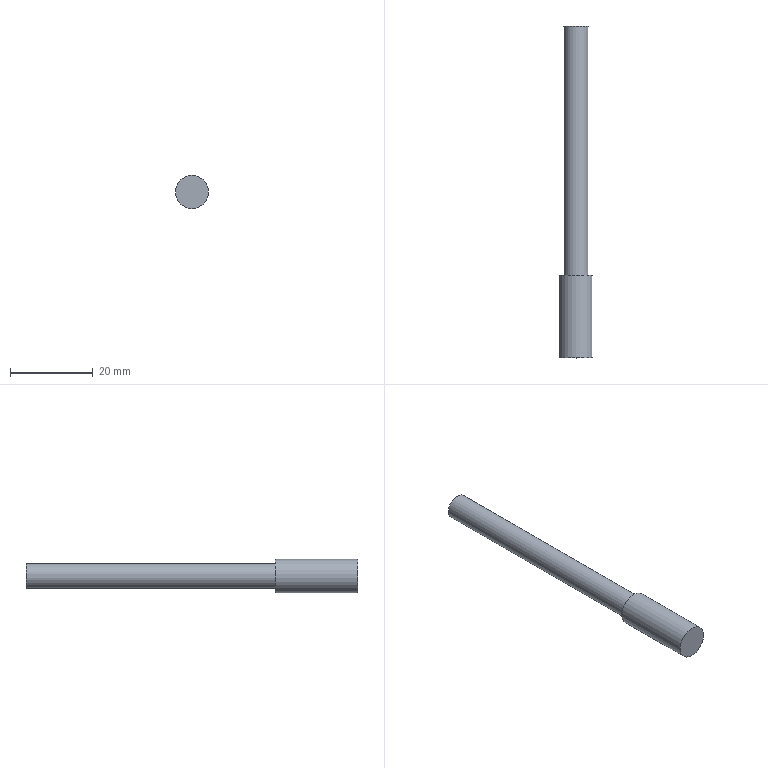Part | NX | features solid 2 | 1 solid | 5 faces | box 8 x 80 x 8 mm | volume 2700 mm3 | plane 3 | cylinder 2 | commonest cylinder face diameters 6 x1 8 x1
STEP:
#1=CARTESIAN_POINT('',(63.5,29.5,7.));
#2=VERTEX_POINT('',#1);
#3=CARTESIAN_POINT('',(63.5,29.5,4.));
#4=DIRECTION('',(0.,1.,0.));
#5=DIRECTION('',(0.,0.,1.));
#6=AXIS2_PLACEMENT_3D('',#3,#4,#5);
#7=CIRCLE('',#6,3.);
#8=EDGE_CURVE('',#2,#2,#7,.F.);
#9=ORIENTED_EDGE('',*,*,#8,.T.);
#10=EDGE_LOOP('',(#9));
#11=FACE_BOUND('',#10,.T.);
#12=CARTESIAN_POINT('',(63.5,-30.6,1.));
#13=VERTEX_POINT('',#12);
#14=CARTESIAN_POINT('',(63.5,-30.6,4.));
#15=DIRECTION('',(0.,-1.,0.));
#16=DIRECTION('',(0.,0.,-1.));
#17=AXIS2_PLACEMENT_3D('',#14,#15,#16);
#18=CIRCLE('',#17,3.);
#19=EDGE_CURVE('',#13,#13,#18,.F.);
#20=ORIENTED_EDGE('',*,*,#19,.T.);
#21=EDGE_LOOP('',(#20));
#22=FACE_BOUND('',#21,.T.);
#23=CARTESIAN_POINT('',(63.5,-69.,4.));
#24=DIRECTION('',(0.,1.,0.));
#25=DIRECTION('',(1.,0.,0.));
#26=AXIS2_PLACEMENT_3D('',#23,#24,#25);
#27=CYLINDRICAL_SURFACE('',#26,3.);
#28=ADVANCED_FACE('',(#11,#22),#27,.T.);
#29=ORIENTED_EDGE('',*,*,#8,.F.);
#30=EDGE_LOOP('',(#29));
#31=FACE_BOUND('',#30,.T.);
#32=CARTESIAN_POINT('',(59.,29.5,-11.));
#33=DIRECTION('',(0.,1.,0.));
#34=DIRECTION('',(0.,0.,1.));
#35=AXIS2_PLACEMENT_3D('',#32,#33,#34);
#36=PLANE('',#35);
#37=ADVANCED_FACE('',(#31),#36,.T.);
#38=CARTESIAN_POINT('',(63.5,-30.6,0.));
#39=VERTEX_POINT('',#38);
#40=CARTESIAN_POINT('',(63.5,-30.6,4.));
#41=DIRECTION('',(0.,-1.,0.));
#42=DIRECTION('',(0.,0.,-1.));
#43=AXIS2_PLACEMENT_3D('',#40,#41,#42);
#44=CIRCLE('',#43,4.);
#45=EDGE_CURVE('',#39,#39,#44,.T.);
#46=ORIENTED_EDGE('',*,*,#45,.T.);
#47=EDGE_LOOP('',(#46));
#48=FACE_BOUND('',#47,.T.);
#49=CARTESIAN_POINT('',(63.5,-50.5,0.));
#50=VERTEX_POINT('',#49);
#51=CARTESIAN_POINT('',(63.5,-50.5,4.));
#52=DIRECTION('',(0.,-1.,0.));
#53=DIRECTION('',(0.,0.,-1.));
#54=AXIS2_PLACEMENT_3D('',#51,#52,#53);
#55=CIRCLE('',#54,4.);
#56=EDGE_CURVE('',#50,#50,#55,.T.);
#57=ORIENTED_EDGE('',*,*,#56,.F.);
#58=EDGE_LOOP('',(#57));
#59=FACE_BOUND('',#58,.T.);
#60=CARTESIAN_POINT('',(63.5,-28.5,4.));
#61=DIRECTION('',(0.,-1.,0.));
#62=DIRECTION('',(0.,0.,-1.));
#63=AXIS2_PLACEMENT_3D('',#60,#61,#62);
#64=CYLINDRICAL_SURFACE('',#63,4.);
#65=ADVANCED_FACE('',(#48,#59),#64,.T.);
#66=ORIENTED_EDGE('',*,*,#19,.F.);
#67=EDGE_LOOP('',(#66));
#68=FACE_BOUND('',#67,.T.);
#69=ORIENTED_EDGE('',*,*,#45,.F.);
#70=EDGE_LOOP('',(#69));
#71=FACE_BOUND('',#70,.T.);
#72=CARTESIAN_POINT('',(63.5,-30.6,4.));
#73=DIRECTION('',(0.,-1.,0.));
#74=DIRECTION('',(0.,0.,-1.));
#75=AXIS2_PLACEMENT_3D('',#72,#73,#74);
#76=PLANE('',#75);
#77=ADVANCED_FACE('',(#68,#71),#76,.F.);
#78=ORIENTED_EDGE('',*,*,#56,.T.);
#79=EDGE_LOOP('',(#78));
#80=FACE_BOUND('',#79,.T.);
#81=CARTESIAN_POINT('',(59.,-50.5,-11.));
#82=DIRECTION('',(0.,-1.,0.));
#83=DIRECTION('',(0.,0.,1.));
#84=AXIS2_PLACEMENT_3D('',#81,#82,#83);
#85=PLANE('',#84);
#86=ADVANCED_FACE('',(#80),#85,.T.);
#87=CLOSED_SHELL('',(#28,#37,#65,#77,#86));
#88=MANIFOLD_SOLID_BREP('',#87);
#89=(LENGTH_UNIT()NAMED_UNIT(*)SI_UNIT(.MILLI.,.METRE.));
#90=UNCERTAINTY_MEASURE_WITH_UNIT(LENGTH_MEASURE(0.00001),#89,'','');
#91=(NAMED_UNIT(*)PLANE_ANGLE_UNIT()SI_UNIT($,.RADIAN.));
#92=(NAMED_UNIT(*)SI_UNIT($,.STERADIAN.)SOLID_ANGLE_UNIT());
#93=(GEOMETRIC_REPRESENTATION_CONTEXT(3)GLOBAL_UNCERTAINTY_ASSIGNED_CONTEXT((#90))GLOBAL_UNIT_ASSIGNED_CONTEXT((#89,#91,#92))REPRESENTATION_CONTEXT('',''));
#94=ADVANCED_BREP_SHAPE_REPRESENTATION('',(#88),#93);